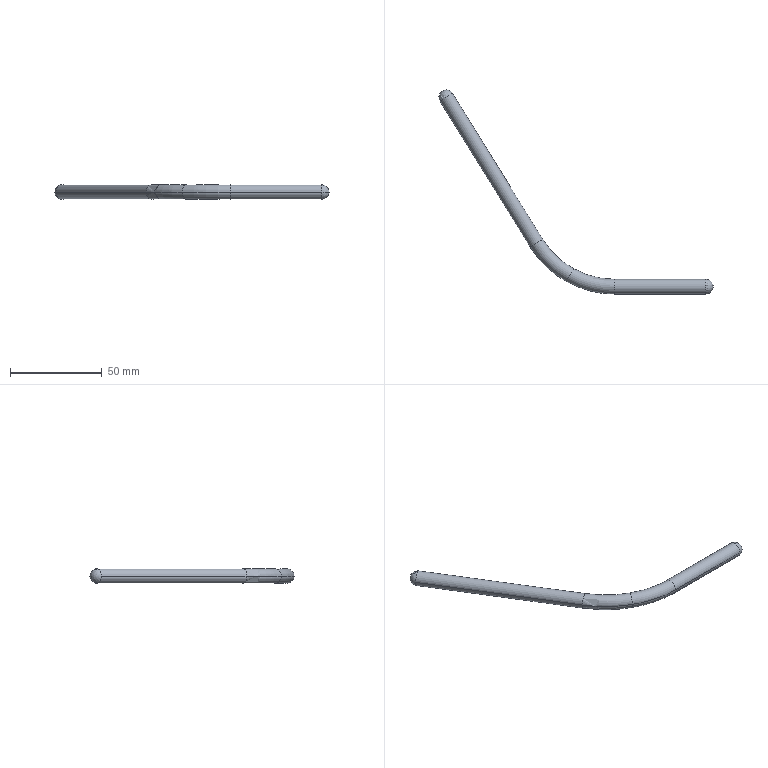Part | Creo | 1 solid | 11 faces | box 149.273 x 111.096 x 8 mm | volume 10012 mm3 | cylinder 4 | torus 4 | sphere 3 | commonest cylinder face diameters 8 x4
STEP:
#1=CARTESIAN_POINT('',(3.963,-14.01,38.161));
#2=VERTEX_POINT('',#1);
#3=CARTESIAN_POINT('',(10.767,-9.802,38.161));
#4=VERTEX_POINT('',#3);
#5=CARTESIAN_POINT('',(7.365,-11.906,38.161));
#6=DIRECTION('',(-0.5261,0.8504,0.));
#7=DIRECTION('',(-0.8504,-0.5261,0.));
#8=AXIS2_PLACEMENT_3D('',#5,#6,#7);
#9=CIRCLE('',#8,4.);
#10=EDGE_CURVE('',#2,#4,#9,.T.);
#11=ORIENTED_EDGE('',*,*,#10,.T.);
#12=CARTESIAN_POINT('',(59.882,-89.201,38.161));
#13=VERTEX_POINT('',#12);
#14=CARTESIAN_POINT('',(59.882,-89.201,38.161));
#15=DIRECTION('',(-0.5261,0.8504,0.));
#16=VECTOR('',#15,93.362);
#17=LINE('',#14,#16);
#18=EDGE_CURVE('',#13,#4,#17,.T.);
#19=ORIENTED_EDGE('',*,*,#18,.F.);
#20=CARTESIAN_POINT('',(53.078,-93.41,38.161));
#21=VERTEX_POINT('',#20);
#22=CARTESIAN_POINT('',(56.48,-91.306,38.161));
#23=DIRECTION('',(0.5261,-0.8504,0.));
#24=DIRECTION('',(0.8504,0.5261,0.));
#25=AXIS2_PLACEMENT_3D('',#22,#23,#24);
#26=CIRCLE('',#25,4.);
#27=EDGE_CURVE('',#13,#21,#26,.T.);
#28=ORIENTED_EDGE('',*,*,#27,.T.);
#29=CARTESIAN_POINT('',(53.078,-93.41,38.161));
#30=DIRECTION('',(-0.5261,0.8504,0.));
#31=VECTOR('',#30,93.362);
#32=LINE('',#29,#31);
#33=EDGE_CURVE('',#21,#2,#32,.T.);
#34=ORIENTED_EDGE('',*,*,#33,.T.);
#35=EDGE_LOOP('',(#11,#19,#28,#34));
#36=FACE_OUTER_BOUND('',#35,.F.);
#37=CARTESIAN_POINT('',(56.48,-91.306,38.161));
#38=DIRECTION('',(-0.5261,0.8504,0.));
#39=DIRECTION('',(-0.8504,-0.5261,0.));
#40=AXIS2_PLACEMENT_3D('',#37,#38,#39);
#41=CYLINDRICAL_SURFACE('',#40,4.);
#42=ADVANCED_FACE('',(#36),#41,.T.);
#43=ORIENTED_EDGE('',*,*,#10,.F.);
#44=CARTESIAN_POINT('',(7.365,-11.906,38.161));
#45=DIRECTION('',(-0.5261,0.8504,0.));
#46=DIRECTION('',(0.8504,0.5261,0.));
#47=AXIS2_PLACEMENT_3D('',#44,#45,#46);
#48=CIRCLE('',#47,4.);
#49=EDGE_CURVE('',#4,#2,#48,.T.);
#50=ORIENTED_EDGE('',*,*,#49,.F.);
#51=EDGE_LOOP('',(#43,#50));
#52=FACE_OUTER_BOUND('',#51,.F.);
#53=CARTESIAN_POINT('',(7.365,-11.906,38.161));
#54=DIRECTION('',(-0.8504,-0.5261,0.));
#55=DIRECTION('',(0.2767,-0.4474,0.8504));
#56=AXIS2_PLACEMENT_3D('',#53,#54,#55);
#57=SPHERICAL_SURFACE('',#56,4.);
#58=ADVANCED_FACE('',(#52),#57,.T.);
#59=ORIENTED_EDGE('',*,*,#49,.T.);
#60=ORIENTED_EDGE('',*,*,#33,.F.);
#61=CARTESIAN_POINT('',(56.48,-91.306,38.161));
#62=DIRECTION('',(0.5261,-0.8504,0.));
#63=DIRECTION('',(-0.8504,-0.5261,0.));
#64=AXIS2_PLACEMENT_3D('',#61,#62,#63);
#65=CIRCLE('',#64,4.);
#66=EDGE_CURVE('',#21,#13,#65,.T.);
#67=ORIENTED_EDGE('',*,*,#66,.T.);
#68=ORIENTED_EDGE('',*,*,#18,.T.);
#69=EDGE_LOOP('',(#59,#60,#67,#68));
#70=FACE_OUTER_BOUND('',#69,.F.);
#71=CARTESIAN_POINT('',(56.48,-91.306,38.161));
#72=DIRECTION('',(-0.5261,0.8504,0.));
#73=DIRECTION('',(-0.8504,-0.5261,0.));
#74=AXIS2_PLACEMENT_3D('',#71,#72,#73);
#75=CYLINDRICAL_SURFACE('',#74,4.);
#76=ADVANCED_FACE('',(#70),#75,.T.);
#77=ORIENTED_EDGE('',*,*,#66,.F.);
#78=CARTESIAN_POINT('',(72.715,-112.172,38.161));
#79=VERTEX_POINT('',#78);
#80=CARTESIAN_POINT('',(99.002,-65.002,38.161));
#81=DIRECTION('',(0.,0.,-1.));
#82=DIRECTION('',(-0.4868,-0.8735,0.));
#83=AXIS2_PLACEMENT_3D('',#80,#81,#82);
#84=CIRCLE('',#83,54.);
#85=EDGE_CURVE('',#79,#21,#84,.T.);
#86=ORIENTED_EDGE('',*,*,#85,.F.);
#87=CARTESIAN_POINT('',(76.609,-105.184,38.161));
#88=VERTEX_POINT('',#87);
#89=CARTESIAN_POINT('',(74.662,-108.678,38.161));
#90=DIRECTION('',(0.8735,-0.4868,0.));
#91=DIRECTION('',(-0.4868,-0.8735,0.));
#92=AXIS2_PLACEMENT_3D('',#89,#90,#91);
#93=CIRCLE('',#92,4.);
#94=EDGE_CURVE('',#79,#88,#93,.T.);
#95=ORIENTED_EDGE('',*,*,#94,.T.);
#96=CARTESIAN_POINT('',(99.002,-65.002,38.161));
#97=DIRECTION('',(0.,0.,-1.));
#98=DIRECTION('',(-0.4868,-0.8735,0.));
#99=AXIS2_PLACEMENT_3D('',#96,#97,#98);
#100=CIRCLE('',#99,46.);
#101=EDGE_CURVE('',#88,#13,#100,.T.);
#102=ORIENTED_EDGE('',*,*,#101,.T.);
#103=EDGE_LOOP('',(#77,#86,#95,#102));
#104=FACE_OUTER_BOUND('',#103,.F.);
#105=CARTESIAN_POINT('',(99.002,-65.002,38.161));
#106=DIRECTION('',(0.,0.,-1.));
#107=DIRECTION('',(-1.,0.,0.));
#108=AXIS2_PLACEMENT_3D('',#105,#106,#107);
#109=TOROIDAL_SURFACE('',#108,50.,4.);
#110=ADVANCED_FACE('',(#104),#109,.T.);
#111=ORIENTED_EDGE('',*,*,#27,.F.);
#112=ORIENTED_EDGE('',*,*,#101,.F.);
#113=CARTESIAN_POINT('',(74.662,-108.678,38.161));
#114=DIRECTION('',(0.8735,-0.4868,0.));
#115=DIRECTION('',(0.4868,0.8735,0.));
#116=AXIS2_PLACEMENT_3D('',#113,#114,#115);
#117=CIRCLE('',#116,4.);
#118=EDGE_CURVE('',#88,#79,#117,.T.);
#119=ORIENTED_EDGE('',*,*,#118,.T.);
#120=ORIENTED_EDGE('',*,*,#85,.T.);
#121=EDGE_LOOP('',(#111,#112,#119,#120));
#122=FACE_OUTER_BOUND('',#121,.F.);
#123=CARTESIAN_POINT('',(99.002,-65.002,38.161));
#124=DIRECTION('',(0.,0.,-1.));
#125=DIRECTION('',(-1.,0.,0.));
#126=AXIS2_PLACEMENT_3D('',#123,#124,#125);
#127=TOROIDAL_SURFACE('',#126,50.,4.);
#128=ADVANCED_FACE('',(#122),#127,.T.);
#129=CARTESIAN_POINT('',(99.002,-119.002,38.161));
#130=VERTEX_POINT('',#129);
#131=CARTESIAN_POINT('',(99.002,-111.002,38.161));
#132=VERTEX_POINT('',#131);
#133=CARTESIAN_POINT('',(99.002,-115.002,38.161));
#134=DIRECTION('',(-1.,0.,0.));
#135=DIRECTION('',(0.,-1.,0.));
#136=AXIS2_PLACEMENT_3D('',#133,#134,#135);
#137=CIRCLE('',#136,4.);
#138=EDGE_CURVE('',#130,#132,#137,.T.);
#139=ORIENTED_EDGE('',*,*,#138,.F.);
#140=CARTESIAN_POINT('',(99.002,-65.002,38.161));
#141=DIRECTION('',(0.,0.,-1.));
#142=DIRECTION('',(0.,-1.,0.));
#143=AXIS2_PLACEMENT_3D('',#140,#141,#142);
#144=CIRCLE('',#143,54.);
#145=EDGE_CURVE('',#130,#79,#144,.T.);
#146=ORIENTED_EDGE('',*,*,#145,.T.);
#147=ORIENTED_EDGE('',*,*,#118,.F.);
#148=CARTESIAN_POINT('',(99.002,-65.002,38.161));
#149=DIRECTION('',(0.,0.,-1.));
#150=DIRECTION('',(0.,-1.,0.));
#151=AXIS2_PLACEMENT_3D('',#148,#149,#150);
#152=CIRCLE('',#151,46.);
#153=EDGE_CURVE('',#132,#88,#152,.T.);
#154=ORIENTED_EDGE('',*,*,#153,.F.);
#155=EDGE_LOOP('',(#139,#146,#147,#154));
#156=FACE_OUTER_BOUND('',#155,.F.);
#157=CARTESIAN_POINT('',(99.002,-65.002,38.161));
#158=DIRECTION('',(0.,0.,-1.));
#159=DIRECTION('',(-1.,0.,0.));
#160=AXIS2_PLACEMENT_3D('',#157,#158,#159);
#161=TOROIDAL_SURFACE('',#160,50.,4.);
#162=ADVANCED_FACE('',(#156),#161,.T.);
#163=CARTESIAN_POINT('',(148.638,-111.002,38.161));
#164=VERTEX_POINT('',#163);
#165=CARTESIAN_POINT('',(148.638,-119.002,38.161));
#166=VERTEX_POINT('',#165);
#167=CARTESIAN_POINT('',(148.638,-115.002,38.161));
#168=DIRECTION('',(1.,0.,0.));
#169=DIRECTION('',(0.,1.,0.));
#170=AXIS2_PLACEMENT_3D('',#167,#168,#169);
#171=CIRCLE('',#170,4.);
#172=EDGE_CURVE('',#164,#166,#171,.T.);
#173=ORIENTED_EDGE('',*,*,#172,.T.);
#174=CARTESIAN_POINT('',(99.002,-119.002,38.161));
#175=DIRECTION('',(1.,0.,0.));
#176=VECTOR('',#175,49.636);
#177=LINE('',#174,#176);
#178=EDGE_CURVE('',#130,#166,#177,.T.);
#179=ORIENTED_EDGE('',*,*,#178,.F.);
#180=ORIENTED_EDGE('',*,*,#138,.T.);
#181=CARTESIAN_POINT('',(99.002,-111.002,38.161));
#182=DIRECTION('',(1.,0.,0.));
#183=VECTOR('',#182,49.636);
#184=LINE('',#181,#183);
#185=EDGE_CURVE('',#132,#164,#184,.T.);
#186=ORIENTED_EDGE('',*,*,#185,.T.);
#187=EDGE_LOOP('',(#173,#179,#180,#186));
#188=FACE_OUTER_BOUND('',#187,.F.);
#189=CARTESIAN_POINT('',(99.002,-115.002,38.161));
#190=DIRECTION('',(1.,0.,0.));
#191=DIRECTION('',(0.,1.,0.));
#192=AXIS2_PLACEMENT_3D('',#189,#190,#191);
#193=CYLINDRICAL_SURFACE('',#192,4.);
#194=ADVANCED_FACE('',(#188),#193,.T.);
#195=ORIENTED_EDGE('',*,*,#172,.F.);
#196=CARTESIAN_POINT('',(148.638,-115.002,38.161));
#197=DIRECTION('',(0.,0.,1.));
#198=DIRECTION('',(0.,-1.,0.));
#199=AXIS2_PLACEMENT_3D('',#196,#197,#198);
#200=CIRCLE('',#199,4.);
#201=EDGE_CURVE('',#166,#164,#200,.T.);
#202=ORIENTED_EDGE('',*,*,#201,.F.);
#203=EDGE_LOOP('',(#195,#202));
#204=FACE_OUTER_BOUND('',#203,.F.);
#205=CARTESIAN_POINT('',(148.638,-115.002,38.161));
#206=DIRECTION('',(0.,1.,0.));
#207=DIRECTION('',(1.,0.,0.));
#208=AXIS2_PLACEMENT_3D('',#205,#206,#207);
#209=SPHERICAL_SURFACE('',#208,4.);
#210=ADVANCED_FACE('',(#204),#209,.T.);
#211=CARTESIAN_POINT('',(148.638,-115.002,38.161));
#212=DIRECTION('',(1.,0.,0.));
#213=DIRECTION('',(0.,-1.,0.));
#214=AXIS2_PLACEMENT_3D('',#211,#212,#213);
#215=CIRCLE('',#214,4.);
#216=EDGE_CURVE('',#166,#164,#215,.T.);
#217=ORIENTED_EDGE('',*,*,#216,.F.);
#218=ORIENTED_EDGE('',*,*,#201,.T.);
#219=EDGE_LOOP('',(#217,#218));
#220=FACE_OUTER_BOUND('',#219,.F.);
#221=CARTESIAN_POINT('',(148.638,-115.002,38.161));
#222=DIRECTION('',(0.,1.,0.));
#223=DIRECTION('',(1.,0.,0.));
#224=AXIS2_PLACEMENT_3D('',#221,#222,#223);
#225=SPHERICAL_SURFACE('',#224,4.);
#226=ADVANCED_FACE('',(#220),#225,.T.);
#227=ORIENTED_EDGE('',*,*,#216,.T.);
#228=ORIENTED_EDGE('',*,*,#185,.F.);
#229=CARTESIAN_POINT('',(99.002,-115.002,38.161));
#230=DIRECTION('',(-1.,0.,0.));
#231=DIRECTION('',(0.,1.,0.));
#232=AXIS2_PLACEMENT_3D('',#229,#230,#231);
#233=CIRCLE('',#232,4.);
#234=EDGE_CURVE('',#132,#130,#233,.T.);
#235=ORIENTED_EDGE('',*,*,#234,.T.);
#236=ORIENTED_EDGE('',*,*,#178,.T.);
#237=EDGE_LOOP('',(#227,#228,#235,#236));
#238=FACE_OUTER_BOUND('',#237,.F.);
#239=CARTESIAN_POINT('',(99.002,-115.002,38.161));
#240=DIRECTION('',(1.,0.,0.));
#241=DIRECTION('',(0.,1.,0.));
#242=AXIS2_PLACEMENT_3D('',#239,#240,#241);
#243=CYLINDRICAL_SURFACE('',#242,4.);
#244=ADVANCED_FACE('',(#238),#243,.T.);
#245=ORIENTED_EDGE('',*,*,#234,.F.);
#246=ORIENTED_EDGE('',*,*,#153,.T.);
#247=ORIENTED_EDGE('',*,*,#94,.F.);
#248=ORIENTED_EDGE('',*,*,#145,.F.);
#249=EDGE_LOOP('',(#245,#246,#247,#248));
#250=FACE_OUTER_BOUND('',#249,.F.);
#251=CARTESIAN_POINT('',(99.002,-65.002,38.161));
#252=DIRECTION('',(0.,0.,-1.));
#253=DIRECTION('',(-1.,0.,0.));
#254=AXIS2_PLACEMENT_3D('',#251,#252,#253);
#255=TOROIDAL_SURFACE('',#254,50.,4.);
#256=ADVANCED_FACE('',(#250),#255,.T.);
#257=CLOSED_SHELL('',(#42,#58,#76,#110,#128,#162,#194,#210,#226,#244,#256));
#258=MANIFOLD_SOLID_BREP('',#257);
#259=(LENGTH_UNIT()NAMED_UNIT(*)SI_UNIT(.MILLI.,.METRE.));
#260=UNCERTAINTY_MEASURE_WITH_UNIT(LENGTH_MEASURE(0.01862),#259,'','');
#261=(NAMED_UNIT(*)PLANE_ANGLE_UNIT()SI_UNIT($,.RADIAN.));
#262=PLANE_ANGLE_MEASURE_WITH_UNIT(PLANE_ANGLE_MEASURE(0.01745),#261);
#263=(CONVERSION_BASED_UNIT('DEGREE',#262)NAMED_UNIT(*)PLANE_ANGLE_UNIT());
#264=(NAMED_UNIT(*)SI_UNIT($,.STERADIAN.)SOLID_ANGLE_UNIT());
#265=(GEOMETRIC_REPRESENTATION_CONTEXT(3)GLOBAL_UNCERTAINTY_ASSIGNED_CONTEXT((#260))GLOBAL_UNIT_ASSIGNED_CONTEXT((#259,#263,#264))REPRESENTATION_CONTEXT('',''));
#266=ADVANCED_BREP_SHAPE_REPRESENTATION('',(#258),#265);